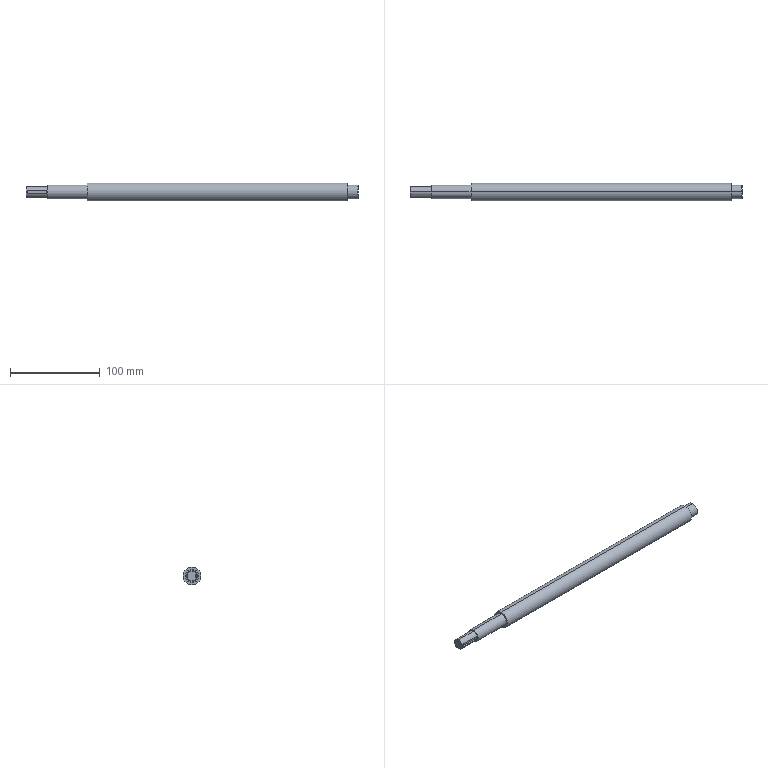Part | SolidWorks | features Chamfer 1, ICE 1, Revolution 1 | 1 solid | 22 faces | box 370 x 20 x 20 mm | volume 103529 mm3 | cylinder 10 | plane 8 | cone 4 | commonest cylinder face diameters 15 x4 4 x2 12 x2 20 x2
STEP:
#1=CARTESIAN_POINT('',(0.,0.,5.5));
#2=VERTEX_POINT('',#1);
#3=CARTESIAN_POINT('',(0.,0.,-5.5));
#4=VERTEX_POINT('',#3);
#5=CARTESIAN_POINT('',(0.,0.,0.));
#6=DIRECTION('',(-1.,0.,0.));
#7=DIRECTION('',(0.,0.,-1.));
#8=AXIS2_PLACEMENT_3D('',#5,#6,#7);
#9=CIRCLE('',#8,5.5);
#10=EDGE_CURVE('',#2,#4,#9,.T.);
#11=ORIENTED_EDGE('',*,*,#10,.F.);
#12=CARTESIAN_POINT('',(0.5,0.,6.));
#13=VERTEX_POINT('',#12);
#14=CARTESIAN_POINT('',(0.,0.,5.5));
#15=DIRECTION('',(0.7071,0.,0.7071));
#16=VECTOR('',#15,1000.);
#17=LINE('',#14,#16);
#18=EDGE_CURVE('',#2,#13,#17,.T.);
#19=ORIENTED_EDGE('',*,*,#18,.T.);
#20=CARTESIAN_POINT('',(0.5,0.,-6.));
#21=VERTEX_POINT('',#20);
#22=CARTESIAN_POINT('',(0.5,0.,0.));
#23=DIRECTION('',(1.,0.,0.));
#24=DIRECTION('',(0.,0.,-1.));
#25=AXIS2_PLACEMENT_3D('',#22,#23,#24);
#26=CIRCLE('',#25,6.);
#27=EDGE_CURVE('',#21,#13,#26,.T.);
#28=ORIENTED_EDGE('',*,*,#27,.F.);
#29=CARTESIAN_POINT('',(0.,0.,-5.5));
#30=DIRECTION('',(0.7071,0.,-0.7071));
#31=VECTOR('',#30,1000.);
#32=LINE('',#29,#31);
#33=EDGE_CURVE('',#4,#21,#32,.T.);
#34=ORIENTED_EDGE('',*,*,#33,.F.);
#35=EDGE_LOOP('',(#11,#19,#28,#34));
#36=FACE_OUTER_BOUND('',#35,.T.);
#37=CARTESIAN_POINT('',(0.,0.,0.));
#38=DIRECTION('',(1.,0.,0.));
#39=DIRECTION('',(0.,0.,-1.));
#40=AXIS2_PLACEMENT_3D('',#37,#38,#39);
#41=CONICAL_SURFACE('',#40,5.5,0.7854);
#42=ADVANCED_FACE('',(#36),#41,.T.);
#43=CARTESIAN_POINT('',(370.,0.,-7.));
#44=VERTEX_POINT('',#43);
#45=CARTESIAN_POINT('',(370.,0.,7.));
#46=VERTEX_POINT('',#45);
#47=CARTESIAN_POINT('',(370.,0.,0.));
#48=DIRECTION('',(1.,0.,0.));
#49=DIRECTION('',(0.,0.,1.));
#50=AXIS2_PLACEMENT_3D('',#47,#48,#49);
#51=CIRCLE('',#50,7.);
#52=EDGE_CURVE('',#44,#46,#51,.T.);
#53=ORIENTED_EDGE('',*,*,#52,.F.);
#54=CARTESIAN_POINT('',(369.5,0.,-7.5));
#55=VERTEX_POINT('',#54);
#56=CARTESIAN_POINT('',(369.5,0.,-7.5));
#57=DIRECTION('',(-0.7071,0.,-0.7071));
#58=VECTOR('',#57,1000.);
#59=LINE('',#56,#58);
#60=EDGE_CURVE('',#44,#55,#59,.T.);
#61=ORIENTED_EDGE('',*,*,#60,.T.);
#62=CARTESIAN_POINT('',(369.5,0.,7.5));
#63=VERTEX_POINT('',#62);
#64=CARTESIAN_POINT('',(369.5,0.,0.));
#65=DIRECTION('',(-1.,0.,0.));
#66=DIRECTION('',(0.,0.,1.));
#67=AXIS2_PLACEMENT_3D('',#64,#65,#66);
#68=CIRCLE('',#67,7.5);
#69=EDGE_CURVE('',#63,#55,#68,.T.);
#70=ORIENTED_EDGE('',*,*,#69,.F.);
#71=CARTESIAN_POINT('',(369.5,0.,7.5));
#72=DIRECTION('',(-0.7071,0.,0.7071));
#73=VECTOR('',#72,1000.);
#74=LINE('',#71,#73);
#75=EDGE_CURVE('',#46,#63,#74,.T.);
#76=ORIENTED_EDGE('',*,*,#75,.F.);
#77=EDGE_LOOP('',(#53,#61,#70,#76));
#78=FACE_OUTER_BOUND('',#77,.T.);
#79=CARTESIAN_POINT('',(369.5,0.,0.));
#80=DIRECTION('',(-1.,0.,0.));
#81=DIRECTION('',(0.,0.,1.));
#82=AXIS2_PLACEMENT_3D('',#79,#80,#81);
#83=CONICAL_SURFACE('',#82,7.5,0.7854);
#84=ADVANCED_FACE('',(#78),#83,.T.);
#85=ORIENTED_EDGE('',*,*,#69,.T.);
#86=CARTESIAN_POINT('',(358.,0.,-7.5));
#87=VERTEX_POINT('',#86);
#88=CARTESIAN_POINT('',(0.,0.,-7.5));
#89=DIRECTION('',(-1.,0.,0.));
#90=VECTOR('',#89,1000.);
#91=LINE('',#88,#90);
#92=EDGE_CURVE('',#55,#87,#91,.T.);
#93=ORIENTED_EDGE('',*,*,#92,.T.);
#94=CARTESIAN_POINT('',(358.,0.,7.5));
#95=VERTEX_POINT('',#94);
#96=CARTESIAN_POINT('',(358.,0.,0.));
#97=DIRECTION('',(-1.,0.,0.));
#98=DIRECTION('',(0.,0.,1.));
#99=AXIS2_PLACEMENT_3D('',#96,#97,#98);
#100=CIRCLE('',#99,7.5);
#101=EDGE_CURVE('',#95,#87,#100,.T.);
#102=ORIENTED_EDGE('',*,*,#101,.F.);
#103=CARTESIAN_POINT('',(0.,0.,7.5));
#104=DIRECTION('',(-1.,0.,0.));
#105=VECTOR('',#104,1000.);
#106=LINE('',#103,#105);
#107=EDGE_CURVE('',#63,#95,#106,.T.);
#108=ORIENTED_EDGE('',*,*,#107,.F.);
#109=EDGE_LOOP('',(#85,#93,#102,#108));
#110=FACE_OUTER_BOUND('',#109,.T.);
#111=CARTESIAN_POINT('',(0.,0.,0.));
#112=DIRECTION('',(-1.,0.,0.));
#113=DIRECTION('',(0.,0.,1.));
#114=AXIS2_PLACEMENT_3D('',#111,#112,#113);
#115=CYLINDRICAL_SURFACE('',#114,7.5);
#116=ADVANCED_FACE('',(#110),#115,.T.);
#117=CARTESIAN_POINT('',(358.,0.,10.));
#118=VERTEX_POINT('',#117);
#119=CARTESIAN_POINT('',(358.,0.,-10.));
#120=VERTEX_POINT('',#119);
#121=CARTESIAN_POINT('',(358.,0.,0.));
#122=DIRECTION('',(-1.,0.,0.));
#123=DIRECTION('',(0.,0.,1.));
#124=AXIS2_PLACEMENT_3D('',#121,#122,#123);
#125=CIRCLE('',#124,10.);
#126=EDGE_CURVE('',#118,#120,#125,.T.);
#127=ORIENTED_EDGE('',*,*,#126,.T.);
#128=CARTESIAN_POINT('',(68.,0.,-10.));
#129=VERTEX_POINT('',#128);
#130=CARTESIAN_POINT('',(0.,0.,-10.));
#131=DIRECTION('',(-1.,0.,0.));
#132=VECTOR('',#131,1000.);
#133=LINE('',#130,#132);
#134=EDGE_CURVE('',#120,#129,#133,.T.);
#135=ORIENTED_EDGE('',*,*,#134,.T.);
#136=CARTESIAN_POINT('',(68.,0.,10.));
#137=VERTEX_POINT('',#136);
#138=CARTESIAN_POINT('',(68.,0.,0.));
#139=DIRECTION('',(-1.,0.,0.));
#140=DIRECTION('',(0.,0.,1.));
#141=AXIS2_PLACEMENT_3D('',#138,#139,#140);
#142=CIRCLE('',#141,10.);
#143=EDGE_CURVE('',#137,#129,#142,.T.);
#144=ORIENTED_EDGE('',*,*,#143,.F.);
#145=CARTESIAN_POINT('',(0.,0.,10.));
#146=DIRECTION('',(-1.,0.,0.));
#147=VECTOR('',#146,1000.);
#148=LINE('',#145,#147);
#149=EDGE_CURVE('',#118,#137,#148,.T.);
#150=ORIENTED_EDGE('',*,*,#149,.F.);
#151=EDGE_LOOP('',(#127,#135,#144,#150));
#152=FACE_OUTER_BOUND('',#151,.T.);
#153=CARTESIAN_POINT('',(0.,0.,0.));
#154=DIRECTION('',(-1.,0.,0.));
#155=DIRECTION('',(0.,0.,1.));
#156=AXIS2_PLACEMENT_3D('',#153,#154,#155);
#157=CYLINDRICAL_SURFACE('',#156,10.);
#158=ADVANCED_FACE('',(#152),#157,.T.);
#159=CARTESIAN_POINT('',(68.,0.,7.5));
#160=VERTEX_POINT('',#159);
#161=CARTESIAN_POINT('',(68.,0.,-7.5));
#162=VERTEX_POINT('',#161);
#163=CARTESIAN_POINT('',(68.,0.,0.));
#164=DIRECTION('',(-1.,0.,0.));
#165=DIRECTION('',(0.,0.,1.));
#166=AXIS2_PLACEMENT_3D('',#163,#164,#165);
#167=CIRCLE('',#166,7.5);
#168=EDGE_CURVE('',#160,#162,#167,.T.);
#169=ORIENTED_EDGE('',*,*,#168,.T.);
#170=CARTESIAN_POINT('',(24.,0.,-7.5));
#171=VERTEX_POINT('',#170);
#172=CARTESIAN_POINT('',(0.,0.,-7.5));
#173=DIRECTION('',(-1.,0.,0.));
#174=VECTOR('',#173,1000.);
#175=LINE('',#172,#174);
#176=EDGE_CURVE('',#162,#171,#175,.T.);
#177=ORIENTED_EDGE('',*,*,#176,.T.);
#178=CARTESIAN_POINT('',(24.,0.,7.5));
#179=VERTEX_POINT('',#178);
#180=CARTESIAN_POINT('',(24.,0.,0.));
#181=DIRECTION('',(-1.,0.,0.));
#182=DIRECTION('',(0.,0.,1.));
#183=AXIS2_PLACEMENT_3D('',#180,#181,#182);
#184=CIRCLE('',#183,7.5);
#185=EDGE_CURVE('',#179,#171,#184,.T.);
#186=ORIENTED_EDGE('',*,*,#185,.F.);
#187=CARTESIAN_POINT('',(0.,0.,7.5));
#188=DIRECTION('',(-1.,0.,0.));
#189=VECTOR('',#188,1000.);
#190=LINE('',#187,#189);
#191=EDGE_CURVE('',#160,#179,#190,.T.);
#192=ORIENTED_EDGE('',*,*,#191,.F.);
#193=EDGE_LOOP('',(#169,#177,#186,#192));
#194=FACE_OUTER_BOUND('',#193,.T.);
#195=CARTESIAN_POINT('',(0.,0.,0.));
#196=DIRECTION('',(-1.,0.,0.));
#197=DIRECTION('',(0.,0.,1.));
#198=AXIS2_PLACEMENT_3D('',#195,#196,#197);
#199=CYLINDRICAL_SURFACE('',#198,7.5);
#200=ADVANCED_FACE('',(#194),#199,.T.);
#201=CARTESIAN_POINT('',(24.,0.,6.));
#202=VERTEX_POINT('',#201);
#203=CARTESIAN_POINT('',(24.,0.,-6.));
#204=VERTEX_POINT('',#203);
#205=CARTESIAN_POINT('',(24.,0.,0.));
#206=DIRECTION('',(-1.,0.,0.));
#207=DIRECTION('',(0.,0.,1.));
#208=AXIS2_PLACEMENT_3D('',#205,#206,#207);
#209=CIRCLE('',#208,6.);
#210=EDGE_CURVE('',#202,#204,#209,.T.);
#211=ORIENTED_EDGE('',*,*,#210,.T.);
#212=CARTESIAN_POINT('',(0.,0.,-6.));
#213=DIRECTION('',(-1.,0.,0.));
#214=VECTOR('',#213,1000.);
#215=LINE('',#212,#214);
#216=EDGE_CURVE('',#204,#21,#215,.T.);
#217=ORIENTED_EDGE('',*,*,#216,.T.);
#218=ORIENTED_EDGE('',*,*,#27,.T.);
#219=CARTESIAN_POINT('',(0.,0.,6.));
#220=DIRECTION('',(-1.,0.,0.));
#221=VECTOR('',#220,1000.);
#222=LINE('',#219,#221);
#223=EDGE_CURVE('',#202,#13,#222,.T.);
#224=ORIENTED_EDGE('',*,*,#223,.F.);
#225=EDGE_LOOP('',(#211,#217,#218,#224));
#226=FACE_OUTER_BOUND('',#225,.T.);
#227=CARTESIAN_POINT('',(0.,0.,0.));
#228=DIRECTION('',(-1.,0.,0.));
#229=DIRECTION('',(0.,0.,1.));
#230=AXIS2_PLACEMENT_3D('',#227,#228,#229);
#231=CYLINDRICAL_SURFACE('',#230,6.);
#232=ADVANCED_FACE('',(#226),#231,.T.);
#233=CARTESIAN_POINT('',(0.,0.,0.));
#234=DIRECTION('',(-1.,0.,0.));
#235=DIRECTION('',(0.,0.,-1.));
#236=AXIS2_PLACEMENT_3D('',#233,#234,#235);
#237=CIRCLE('',#236,5.5);
#238=EDGE_CURVE('',#4,#2,#237,.T.);
#239=ORIENTED_EDGE('',*,*,#238,.T.);
#240=ORIENTED_EDGE('',*,*,#10,.T.);
#241=EDGE_LOOP('',(#239,#240));
#242=FACE_OUTER_BOUND('',#241,.T.);
#243=CARTESIAN_POINT('',(0.,0.,0.));
#244=DIRECTION('',(1.,0.,0.));
#245=DIRECTION('',(0.,0.,-1.));
#246=AXIS2_PLACEMENT_3D('',#243,#244,#245);
#247=PLANE('',#246);
#248=ADVANCED_FACE('',(#242),#247,.F.);
#249=ORIENTED_EDGE('',*,*,#216,.F.);
#250=CARTESIAN_POINT('',(24.,0.,0.));
#251=DIRECTION('',(-1.,0.,0.));
#252=DIRECTION('',(0.,0.,1.));
#253=AXIS2_PLACEMENT_3D('',#250,#251,#252);
#254=CIRCLE('',#253,6.);
#255=EDGE_CURVE('',#204,#202,#254,.T.);
#256=ORIENTED_EDGE('',*,*,#255,.T.);
#257=ORIENTED_EDGE('',*,*,#223,.T.);
#258=CARTESIAN_POINT('',(0.5,0.,0.));
#259=DIRECTION('',(1.,0.,0.));
#260=DIRECTION('',(0.,0.,-1.));
#261=AXIS2_PLACEMENT_3D('',#258,#259,#260);
#262=CIRCLE('',#261,6.);
#263=EDGE_CURVE('',#13,#21,#262,.T.);
#264=ORIENTED_EDGE('',*,*,#263,.T.);
#265=EDGE_LOOP('',(#249,#256,#257,#264));
#266=FACE_OUTER_BOUND('',#265,.T.);
#267=CARTESIAN_POINT('',(21.,-5.657,-2.));
#268=VERTEX_POINT('',#267);
#269=CARTESIAN_POINT('',(3.,-5.657,-2.));
#270=VERTEX_POINT('',#269);
#271=CARTESIAN_POINT('',(0.,-5.657,-2.));
#272=DIRECTION('',(-1.,0.,0.));
#273=VECTOR('',#272,1000.);
#274=LINE('',#271,#273);
#275=EDGE_CURVE('',#268,#270,#274,.T.);
#276=ORIENTED_EDGE('',*,*,#275,.T.);
#277=CARTESIAN_POINT('',(3.,-5.657,2.));
#278=VERTEX_POINT('',#277);
#279=CARTESIAN_POINT('',(3.,-5.657,-2.));
#280=CARTESIAN_POINT('',(2.867,-5.657,-2.));
#281=CARTESIAN_POINT('',(2.736,-5.662,-1.987));
#282=CARTESIAN_POINT('',(2.479,-5.679,-1.935));
#283=CARTESIAN_POINT('',(2.352,-5.693,-1.897));
#284=CARTESIAN_POINT('',(2.11,-5.725,-1.796));
#285=CARTESIAN_POINT('',(1.996,-5.744,-1.735));
#286=CARTESIAN_POINT('',(1.779,-5.786,-1.59));
#287=CARTESIAN_POINT('',(1.677,-5.809,-1.506));
#288=CARTESIAN_POINT('',(1.403,-5.875,-1.231));
#289=CARTESIAN_POINT('',(1.254,-5.919,-1.01));
#290=CARTESIAN_POINT('',(1.104,-5.966,-0.6496));
#291=CARTESIAN_POINT('',(1.065,-5.979,-0.5226));
#292=CARTESIAN_POINT('',(1.013,-5.996,-0.264));
#293=CARTESIAN_POINT('',(1.,-6.,-0.1336));
#294=CARTESIAN_POINT('',(0.9999,-6.,0.1294));
#295=CARTESIAN_POINT('',(1.013,-5.996,0.2629));
#296=CARTESIAN_POINT('',(1.064,-5.979,0.5202));
#297=CARTESIAN_POINT('',(1.102,-5.966,0.6454));
#298=CARTESIAN_POINT('',(1.204,-5.935,0.8889));
#299=CARTESIAN_POINT('',(1.266,-5.916,1.004));
#300=CARTESIAN_POINT('',(1.41,-5.876,1.22));
#301=CARTESIAN_POINT('',(1.493,-5.853,1.322));
#302=CARTESIAN_POINT('',(1.677,-5.809,1.506));
#303=CARTESIAN_POINT('',(1.777,-5.787,1.588));
#304=CARTESIAN_POINT('',(1.993,-5.745,1.733));
#305=CARTESIAN_POINT('',(2.11,-5.725,1.796));
#306=CARTESIAN_POINT('',(2.471,-5.677,1.946));
#307=CARTESIAN_POINT('',(2.734,-5.657,2.));
#308=CARTESIAN_POINT('',(3.,-5.657,2.));
#309=B_SPLINE_CURVE_WITH_KNOTS('',3,(#279,#280,#281,#282,#283,#284,#285,#286,#287,#288,#289,#290,#291,#292,#293,#294,#295,#296,#297,#298,#299,#300,#301,#302,#303,#304,#305,#306,#307,#308),.UNSPECIFIED.,.F.,.F.,(4,2,2,2,2,2,2,2,2,2,2,2,2,2,4),(0.,0.0003935,0.000787,0.00118,0.001574,0.002361,0.002754,0.003148,0.003541,0.003935,0.004328,0.004722,0.005115,0.005509,0.006296),.UNSPECIFIED.);
#310=EDGE_CURVE('',#270,#278,#309,.T.);
#311=ORIENTED_EDGE('',*,*,#310,.T.);
#312=CARTESIAN_POINT('',(21.,-5.657,2.));
#313=VERTEX_POINT('',#312);
#314=CARTESIAN_POINT('',(0.,-5.657,2.));
#315=DIRECTION('',(1.,0.,0.));
#316=VECTOR('',#315,1000.);
#317=LINE('',#314,#316);
#318=EDGE_CURVE('',#278,#313,#317,.T.);
#319=ORIENTED_EDGE('',*,*,#318,.T.);
#320=CARTESIAN_POINT('',(21.,-5.657,2.));
#321=CARTESIAN_POINT('',(21.133,-5.657,2.));
#322=CARTESIAN_POINT('',(21.264,-5.662,1.987));
#323=CARTESIAN_POINT('',(21.521,-5.679,1.935));
#324=CARTESIAN_POINT('',(21.648,-5.693,1.897));
#325=CARTESIAN_POINT('',(21.89,-5.725,1.796));
#326=CARTESIAN_POINT('',(22.004,-5.744,1.735));
#327=CARTESIAN_POINT('',(22.221,-5.786,1.59));
#328=CARTESIAN_POINT('',(22.323,-5.809,1.506));
#329=CARTESIAN_POINT('',(22.597,-5.875,1.231));
#330=CARTESIAN_POINT('',(22.746,-5.919,1.01));
#331=CARTESIAN_POINT('',(22.896,-5.966,0.6496));
#332=CARTESIAN_POINT('',(22.935,-5.979,0.5226));
#333=CARTESIAN_POINT('',(22.987,-5.996,0.264));
#334=CARTESIAN_POINT('',(23.,-6.,0.1336));
#335=CARTESIAN_POINT('',(23.,-6.,-0.1294));
#336=CARTESIAN_POINT('',(22.987,-5.996,-0.2629));
#337=CARTESIAN_POINT('',(22.936,-5.979,-0.5202));
#338=CARTESIAN_POINT('',(22.898,-5.966,-0.6454));
#339=CARTESIAN_POINT('',(22.796,-5.935,-0.8889));
#340=CARTESIAN_POINT('',(22.734,-5.916,-1.004));
#341=CARTESIAN_POINT('',(22.59,-5.876,-1.22));
#342=CARTESIAN_POINT('',(22.507,-5.853,-1.322));
#343=CARTESIAN_POINT('',(22.323,-5.809,-1.506));
#344=CARTESIAN_POINT('',(22.223,-5.787,-1.588));
#345=CARTESIAN_POINT('',(22.007,-5.745,-1.733));
#346=CARTESIAN_POINT('',(21.89,-5.725,-1.796));
#347=CARTESIAN_POINT('',(21.529,-5.677,-1.946));
#348=CARTESIAN_POINT('',(21.266,-5.657,-2.));
#349=CARTESIAN_POINT('',(21.,-5.657,-2.));
#350=B_SPLINE_CURVE_WITH_KNOTS('',3,(#320,#321,#322,#323,#324,#325,#326,#327,#328,#329,#330,#331,#332,#333,#334,#335,#336,#337,#338,#339,#340,#341,#342,#343,#344,#345,#346,#347,#348,#349),.UNSPECIFIED.,.F.,.F.,(4,2,2,2,2,2,2,2,2,2,2,2,2,2,4),(0.,0.0003935,0.000787,0.00118,0.001574,0.002361,0.002754,0.003148,0.003541,0.003935,0.004328,0.004722,0.005115,0.005509,0.006296),.UNSPECIFIED.);
#351=EDGE_CURVE('',#313,#268,#350,.T.);
#352=ORIENTED_EDGE('',*,*,#351,.T.);
#353=EDGE_LOOP('',(#276,#311,#319,#352));
#354=FACE_BOUND('',#353,.T.);
#355=CARTESIAN_POINT('',(0.,0.,0.));
#356=DIRECTION('',(-1.,0.,0.));
#357=DIRECTION('',(0.,0.,1.));
#358=AXIS2_PLACEMENT_3D('',#355,#356,#357);
#359=CYLINDRICAL_SURFACE('',#358,6.);
#360=ADVANCED_FACE('',(#266,#354),#359,.T.);
#361=ORIENTED_EDGE('',*,*,#210,.F.);
#362=ORIENTED_EDGE('',*,*,#255,.F.);
#363=EDGE_LOOP('',(#361,#362));
#364=FACE_BOUND('',#363,.T.);
#365=ORIENTED_EDGE('',*,*,#185,.T.);
#366=CARTESIAN_POINT('',(24.,0.,0.));
#367=DIRECTION('',(-1.,0.,0.));
#368=DIRECTION('',(0.,0.,1.));
#369=AXIS2_PLACEMENT_3D('',#366,#367,#368);
#370=CIRCLE('',#369,7.5);
#371=EDGE_CURVE('',#171,#179,#370,.T.);
#372=ORIENTED_EDGE('',*,*,#371,.T.);
#373=EDGE_LOOP('',(#365,#372));
#374=FACE_OUTER_BOUND('',#373,.T.);
#375=CARTESIAN_POINT('',(24.,0.,-6.));
#376=DIRECTION('',(1.,0.,0.));
#377=DIRECTION('',(0.,0.,-1.));
#378=AXIS2_PLACEMENT_3D('',#375,#376,#377);
#379=PLANE('',#378);
#380=ADVANCED_FACE('',(#364,#374),#379,.F.);
#381=ORIENTED_EDGE('',*,*,#176,.F.);
#382=CARTESIAN_POINT('',(68.,0.,0.));
#383=DIRECTION('',(-1.,0.,0.));
#384=DIRECTION('',(0.,0.,1.));
#385=AXIS2_PLACEMENT_3D('',#382,#383,#384);
#386=CIRCLE('',#385,7.5);
#387=EDGE_CURVE('',#162,#160,#386,.T.);
#388=ORIENTED_EDGE('',*,*,#387,.T.);
#389=ORIENTED_EDGE('',*,*,#191,.T.);
#390=ORIENTED_EDGE('',*,*,#371,.F.);
#391=EDGE_LOOP('',(#381,#388,#389,#390));
#392=FACE_OUTER_BOUND('',#391,.T.);
#393=CARTESIAN_POINT('',(0.,0.,0.));
#394=DIRECTION('',(-1.,0.,0.));
#395=DIRECTION('',(0.,0.,1.));
#396=AXIS2_PLACEMENT_3D('',#393,#394,#395);
#397=CYLINDRICAL_SURFACE('',#396,7.5);
#398=ADVANCED_FACE('',(#392),#397,.T.);
#399=ORIENTED_EDGE('',*,*,#168,.F.);
#400=ORIENTED_EDGE('',*,*,#387,.F.);
#401=EDGE_LOOP('',(#399,#400));
#402=FACE_BOUND('',#401,.T.);
#403=ORIENTED_EDGE('',*,*,#143,.T.);
#404=CARTESIAN_POINT('',(68.,0.,0.));
#405=DIRECTION('',(-1.,0.,0.));
#406=DIRECTION('',(0.,0.,1.));
#407=AXIS2_PLACEMENT_3D('',#404,#405,#406);
#408=CIRCLE('',#407,10.);
#409=EDGE_CURVE('',#129,#137,#408,.T.);
#410=ORIENTED_EDGE('',*,*,#409,.T.);
#411=EDGE_LOOP('',(#403,#410));
#412=FACE_OUTER_BOUND('',#411,.T.);
#413=CARTESIAN_POINT('',(68.,0.,-7.5));
#414=DIRECTION('',(1.,0.,0.));
#415=DIRECTION('',(0.,0.,-1.));
#416=AXIS2_PLACEMENT_3D('',#413,#414,#415);
#417=PLANE('',#416);
#418=ADVANCED_FACE('',(#402,#412),#417,.F.);
#419=ORIENTED_EDGE('',*,*,#134,.F.);
#420=CARTESIAN_POINT('',(358.,0.,0.));
#421=DIRECTION('',(-1.,0.,0.));
#422=DIRECTION('',(0.,0.,1.));
#423=AXIS2_PLACEMENT_3D('',#420,#421,#422);
#424=CIRCLE('',#423,10.);
#425=EDGE_CURVE('',#120,#118,#424,.T.);
#426=ORIENTED_EDGE('',*,*,#425,.T.);
#427=ORIENTED_EDGE('',*,*,#149,.T.);
#428=ORIENTED_EDGE('',*,*,#409,.F.);
#429=EDGE_LOOP('',(#419,#426,#427,#428));
#430=FACE_OUTER_BOUND('',#429,.T.);
#431=CARTESIAN_POINT('',(0.,0.,0.));
#432=DIRECTION('',(-1.,0.,0.));
#433=DIRECTION('',(0.,0.,1.));
#434=AXIS2_PLACEMENT_3D('',#431,#432,#433);
#435=CYLINDRICAL_SURFACE('',#434,10.);
#436=ADVANCED_FACE('',(#430),#435,.T.);
#437=ORIENTED_EDGE('',*,*,#126,.F.);
#438=ORIENTED_EDGE('',*,*,#425,.F.);
#439=EDGE_LOOP('',(#437,#438));
#440=FACE_OUTER_BOUND('',#439,.T.);
#441=ORIENTED_EDGE('',*,*,#101,.T.);
#442=CARTESIAN_POINT('',(358.,0.,0.));
#443=DIRECTION('',(-1.,0.,0.));
#444=DIRECTION('',(0.,0.,1.));
#445=AXIS2_PLACEMENT_3D('',#442,#443,#444);
#446=CIRCLE('',#445,7.5);
#447=EDGE_CURVE('',#87,#95,#446,.T.);
#448=ORIENTED_EDGE('',*,*,#447,.T.);
#449=EDGE_LOOP('',(#441,#448));
#450=FACE_BOUND('',#449,.T.);
#451=CARTESIAN_POINT('',(358.,0.,-10.));
#452=DIRECTION('',(-1.,0.,0.));
#453=DIRECTION('',(0.,0.,1.));
#454=AXIS2_PLACEMENT_3D('',#451,#452,#453);
#455=PLANE('',#454);
#456=ADVANCED_FACE('',(#440,#450),#455,.F.);
#457=ORIENTED_EDGE('',*,*,#92,.F.);
#458=CARTESIAN_POINT('',(369.5,0.,0.));
#459=DIRECTION('',(-1.,0.,0.));
#460=DIRECTION('',(0.,0.,1.));
#461=AXIS2_PLACEMENT_3D('',#458,#459,#460);
#462=CIRCLE('',#461,7.5);
#463=EDGE_CURVE('',#55,#63,#462,.T.);
#464=ORIENTED_EDGE('',*,*,#463,.T.);
#465=ORIENTED_EDGE('',*,*,#107,.T.);
#466=ORIENTED_EDGE('',*,*,#447,.F.);
#467=EDGE_LOOP('',(#457,#464,#465,#466));
#468=FACE_OUTER_BOUND('',#467,.T.);
#469=CARTESIAN_POINT('',(0.,0.,0.));
#470=DIRECTION('',(-1.,0.,0.));
#471=DIRECTION('',(0.,0.,1.));
#472=AXIS2_PLACEMENT_3D('',#469,#470,#471);
#473=CYLINDRICAL_SURFACE('',#472,7.5);
#474=ADVANCED_FACE('',(#468),#473,.T.);
#475=CARTESIAN_POINT('',(370.,0.,0.));
#476=DIRECTION('',(1.,0.,0.));
#477=DIRECTION('',(0.,0.,1.));
#478=AXIS2_PLACEMENT_3D('',#475,#476,#477);
#479=CIRCLE('',#478,7.);
#480=EDGE_CURVE('',#46,#44,#479,.T.);
#481=ORIENTED_EDGE('',*,*,#480,.T.);
#482=ORIENTED_EDGE('',*,*,#52,.T.);
#483=EDGE_LOOP('',(#481,#482));
#484=FACE_OUTER_BOUND('',#483,.T.);
#485=CARTESIAN_POINT('',(370.,0.,-7.5));
#486=DIRECTION('',(-1.,0.,0.));
#487=DIRECTION('',(0.,0.,1.));
#488=AXIS2_PLACEMENT_3D('',#485,#486,#487);
#489=PLANE('',#488);
#490=ADVANCED_FACE('',(#484),#489,.F.);
#491=CARTESIAN_POINT('',(21.,-3.8,2.));
#492=VERTEX_POINT('',#491);
#493=CARTESIAN_POINT('',(21.,-3.8,2.));
#494=DIRECTION('',(0.,-1.,0.));
#495=VECTOR('',#494,1000.);
#496=LINE('',#493,#495);
#497=EDGE_CURVE('',#492,#313,#496,.T.);
#498=ORIENTED_EDGE('',*,*,#497,.F.);
#499=CARTESIAN_POINT('',(21.,-3.8,-2.));
#500=VERTEX_POINT('',#499);
#501=CARTESIAN_POINT('',(21.,-3.8,0.));
#502=DIRECTION('',(0.,-1.,0.));
#503=DIRECTION('',(0.,0.,-1.));
#504=AXIS2_PLACEMENT_3D('',#501,#502,#503);
#505=CIRCLE('',#504,2.);
#506=EDGE_CURVE('',#500,#492,#505,.T.);
#507=ORIENTED_EDGE('',*,*,#506,.F.);
#508=CARTESIAN_POINT('',(21.,-3.8,-2.));
#509=DIRECTION('',(0.,-1.,0.));
#510=VECTOR('',#509,1000.);
#511=LINE('',#508,#510);
#512=EDGE_CURVE('',#500,#268,#511,.T.);
#513=ORIENTED_EDGE('',*,*,#512,.T.);
#514=ORIENTED_EDGE('',*,*,#351,.F.);
#515=EDGE_LOOP('',(#498,#507,#513,#514));
#516=FACE_OUTER_BOUND('',#515,.T.);
#517=CARTESIAN_POINT('',(21.,-3.8,0.));
#518=DIRECTION('',(0.,-1.,0.));
#519=DIRECTION('',(0.,0.,-1.));
#520=AXIS2_PLACEMENT_3D('',#517,#518,#519);
#521=CYLINDRICAL_SURFACE('',#520,2.);
#522=ADVANCED_FACE('',(#516),#521,.F.);
#523=ORIENTED_EDGE('',*,*,#512,.F.);
#524=CARTESIAN_POINT('',(3.,-3.8,-2.));
#525=VERTEX_POINT('',#524);
#526=CARTESIAN_POINT('',(21.,-3.8,-2.));
#527=DIRECTION('',(1.,0.,0.));
#528=VECTOR('',#527,1000.);
#529=LINE('',#526,#528);
#530=EDGE_CURVE('',#525,#500,#529,.T.);
#531=ORIENTED_EDGE('',*,*,#530,.F.);
#532=CARTESIAN_POINT('',(3.,-3.8,-2.));
#533=DIRECTION('',(0.,-1.,0.));
#534=VECTOR('',#533,1000.);
#535=LINE('',#532,#534);
#536=EDGE_CURVE('',#525,#270,#535,.T.);
#537=ORIENTED_EDGE('',*,*,#536,.T.);
#538=ORIENTED_EDGE('',*,*,#275,.F.);
#539=EDGE_LOOP('',(#523,#531,#537,#538));
#540=FACE_OUTER_BOUND('',#539,.T.);
#541=CARTESIAN_POINT('',(21.,-3.8,-2.));
#542=DIRECTION('',(0.,0.,-1.));
#543=DIRECTION('',(-1.,0.,0.));
#544=AXIS2_PLACEMENT_3D('',#541,#542,#543);
#545=PLANE('',#544);
#546=ADVANCED_FACE('',(#540),#545,.F.);
#547=ORIENTED_EDGE('',*,*,#536,.F.);
#548=CARTESIAN_POINT('',(3.,-3.8,2.));
#549=VERTEX_POINT('',#548);
#550=CARTESIAN_POINT('',(3.,-3.8,0.));
#551=DIRECTION('',(0.,-1.,0.));
#552=DIRECTION('',(0.,0.,-1.));
#553=AXIS2_PLACEMENT_3D('',#550,#551,#552);
#554=CIRCLE('',#553,2.);
#555=EDGE_CURVE('',#549,#525,#554,.T.);
#556=ORIENTED_EDGE('',*,*,#555,.F.);
#557=CARTESIAN_POINT('',(3.,-3.8,2.));
#558=DIRECTION('',(0.,-1.,0.));
#559=VECTOR('',#558,1000.);
#560=LINE('',#557,#559);
#561=EDGE_CURVE('',#549,#278,#560,.T.);
#562=ORIENTED_EDGE('',*,*,#561,.T.);
#563=ORIENTED_EDGE('',*,*,#310,.F.);
#564=EDGE_LOOP('',(#547,#556,#562,#563));
#565=FACE_OUTER_BOUND('',#564,.T.);
#566=CARTESIAN_POINT('',(3.,-3.8,0.));
#567=DIRECTION('',(0.,-1.,0.));
#568=DIRECTION('',(0.,0.,-1.));
#569=AXIS2_PLACEMENT_3D('',#566,#567,#568);
#570=CYLINDRICAL_SURFACE('',#569,2.);
#571=ADVANCED_FACE('',(#565),#570,.F.);
#572=ORIENTED_EDGE('',*,*,#561,.F.);
#573=CARTESIAN_POINT('',(21.,-3.8,2.));
#574=DIRECTION('',(-1.,0.,0.));
#575=VECTOR('',#574,1000.);
#576=LINE('',#573,#575);
#577=EDGE_CURVE('',#492,#549,#576,.T.);
#578=ORIENTED_EDGE('',*,*,#577,.F.);
#579=ORIENTED_EDGE('',*,*,#497,.T.);
#580=ORIENTED_EDGE('',*,*,#318,.F.);
#581=EDGE_LOOP('',(#572,#578,#579,#580));
#582=FACE_OUTER_BOUND('',#581,.T.);
#583=CARTESIAN_POINT('',(21.,-3.8,2.));
#584=DIRECTION('',(0.,0.,1.));
#585=DIRECTION('',(1.,0.,0.));
#586=AXIS2_PLACEMENT_3D('',#583,#584,#585);
#587=PLANE('',#586);
#588=ADVANCED_FACE('',(#582),#587,.F.);
#589=ORIENTED_EDGE('',*,*,#506,.T.);
#590=ORIENTED_EDGE('',*,*,#577,.T.);
#591=ORIENTED_EDGE('',*,*,#555,.T.);
#592=ORIENTED_EDGE('',*,*,#530,.T.);
#593=EDGE_LOOP('',(#589,#590,#591,#592));
#594=FACE_OUTER_BOUND('',#593,.T.);
#595=CARTESIAN_POINT('',(21.,-3.8,0.));
#596=DIRECTION('',(0.,-1.,0.));
#597=DIRECTION('',(0.,0.,-1.));
#598=AXIS2_PLACEMENT_3D('',#595,#596,#597);
#599=PLANE('',#598);
#600=ADVANCED_FACE('',(#594),#599,.T.);
#601=ORIENTED_EDGE('',*,*,#60,.F.);
#602=ORIENTED_EDGE('',*,*,#480,.F.);
#603=ORIENTED_EDGE('',*,*,#75,.T.);
#604=ORIENTED_EDGE('',*,*,#463,.F.);
#605=EDGE_LOOP('',(#601,#602,#603,#604));
#606=FACE_OUTER_BOUND('',#605,.T.);
#607=CARTESIAN_POINT('',(369.5,0.,0.));
#608=DIRECTION('',(-1.,0.,0.));
#609=DIRECTION('',(0.,0.,1.));
#610=AXIS2_PLACEMENT_3D('',#607,#608,#609);
#611=CONICAL_SURFACE('',#610,7.5,0.7854);
#612=ADVANCED_FACE('',(#606),#611,.T.);
#613=ORIENTED_EDGE('',*,*,#18,.F.);
#614=ORIENTED_EDGE('',*,*,#238,.F.);
#615=ORIENTED_EDGE('',*,*,#33,.T.);
#616=ORIENTED_EDGE('',*,*,#263,.F.);
#617=EDGE_LOOP('',(#613,#614,#615,#616));
#618=FACE_OUTER_BOUND('',#617,.T.);
#619=CARTESIAN_POINT('',(0.,0.,0.));
#620=DIRECTION('',(1.,0.,0.));
#621=DIRECTION('',(0.,0.,-1.));
#622=AXIS2_PLACEMENT_3D('',#619,#620,#621);
#623=CONICAL_SURFACE('',#622,5.5,0.7854);
#624=ADVANCED_FACE('',(#618),#623,.T.);
#625=CLOSED_SHELL('',(#42,#84,#116,#158,#200,#232,#248,#360,#380,#398,#418,#436,#456,#474,#490,#522,#546,#571,#588,#600,#612,#624));
#626=MANIFOLD_SOLID_BREP('',#625);
#627=CARTESIAN_POINT('',(0.,0.,0.));
#628=DIRECTION('',(0.,0.,1.));
#629=DIRECTION('',(1.,0.,0.));
#630=AXIS2_PLACEMENT_3D('',#627,#628,#629);
#631=(LENGTH_UNIT()NAMED_UNIT(*)SI_UNIT(.MILLI.,.METRE.));
#632=UNCERTAINTY_MEASURE_WITH_UNIT(LENGTH_MEASURE(0.00001),#631,'','');
#633=(NAMED_UNIT(*)PLANE_ANGLE_UNIT()SI_UNIT($,.RADIAN.));
#634=(NAMED_UNIT(*)SI_UNIT($,.STERADIAN.)SOLID_ANGLE_UNIT());
#635=(GEOMETRIC_REPRESENTATION_CONTEXT(3)GLOBAL_UNCERTAINTY_ASSIGNED_CONTEXT((#632))GLOBAL_UNIT_ASSIGNED_CONTEXT((#631,#633,#634))REPRESENTATION_CONTEXT('',''));
#636=ADVANCED_BREP_SHAPE_REPRESENTATION('',(#626,#630),#635);